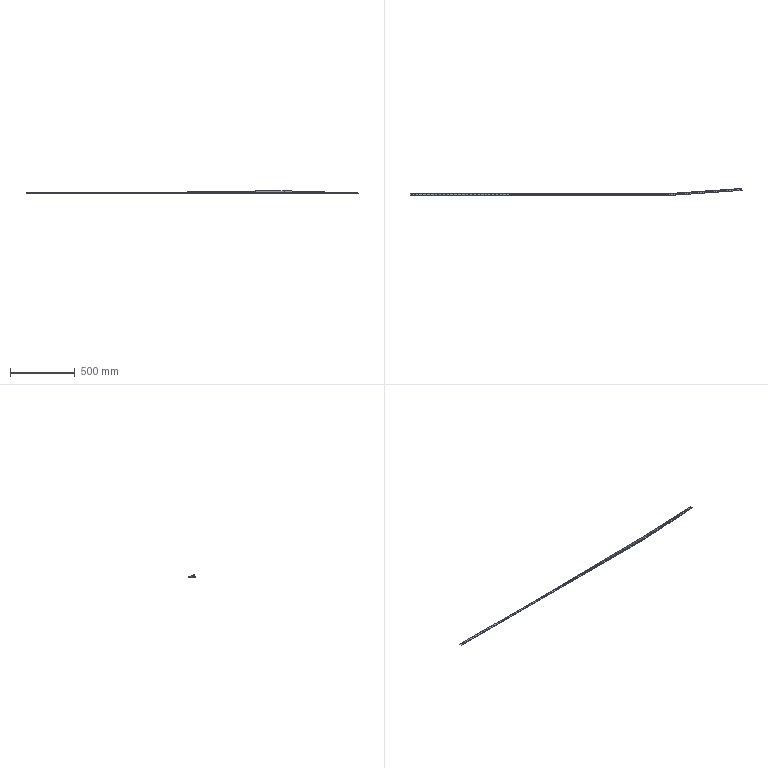Part | SolidWorks | features BaseBody 1 | 1 solid | 232 faces | box 2573 x 55.001 x 21.062 mm | volume 169917 mm3 | cylinder 220 | plane 12 | commonest cylinder face diameters 3.2 x220